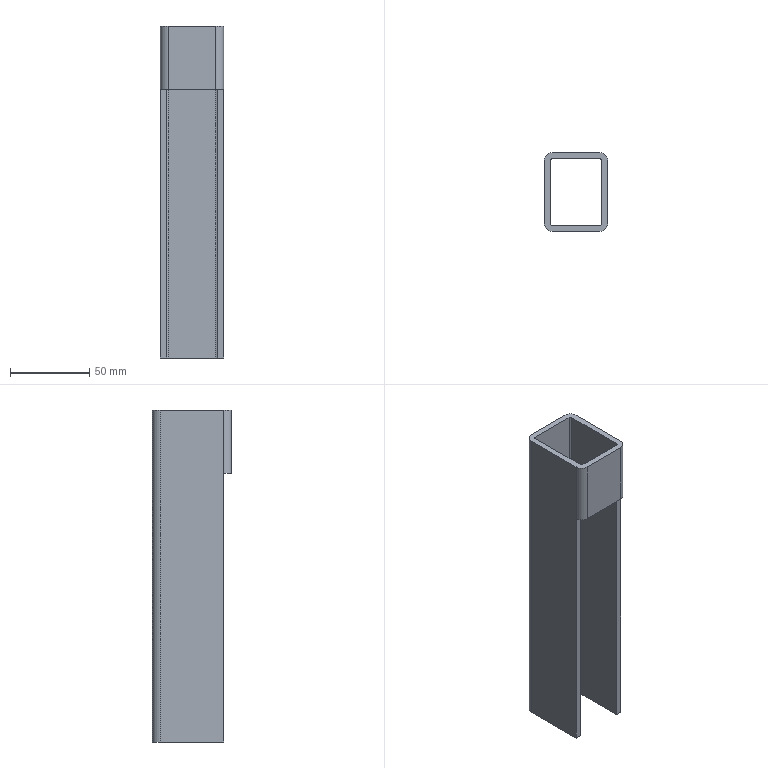Part | SolidWorks | features BaseBody 1 | 1 solid | 21 faces | box 40 x 50 x 210 mm | volume 100329 mm3 | plane 13 | cylinder 8 | commonest cylinder face diameters 2.5 x4 10 x4
STEP:
#1=CARTESIAN_POINT('',(20.,-20.,65.));
#2=VERTEX_POINT('',#1);
#3=CARTESIAN_POINT('',(20.,-20.,-105.));
#4=VERTEX_POINT('',#3);
#5=CARTESIAN_POINT('',(20.,-20.,-115.));
#6=DIRECTION('',(0.,0.,-1.));
#7=VECTOR('',#6,1000.);
#8=LINE('',#5,#7);
#9=EDGE_CURVE('',#2,#4,#8,.T.);
#10=ORIENTED_EDGE('',*,*,#9,.F.);
#11=CARTESIAN_POINT('',(16.25,-20.,65.));
#12=VERTEX_POINT('',#11);
#13=CARTESIAN_POINT('',(20.,-20.,65.));
#14=DIRECTION('',(-1.,0.,0.));
#15=VECTOR('',#14,1000.);
#16=LINE('',#13,#15);
#17=EDGE_CURVE('',#2,#12,#16,.T.);
#18=ORIENTED_EDGE('',*,*,#17,.T.);
#19=CARTESIAN_POINT('',(16.25,-20.,-105.));
#20=VERTEX_POINT('',#19);
#21=CARTESIAN_POINT('',(16.25,-20.,105.));
#22=DIRECTION('',(0.,0.,-1.));
#23=VECTOR('',#22,1000.);
#24=LINE('',#21,#23);
#25=EDGE_CURVE('',#12,#20,#24,.T.);
#26=ORIENTED_EDGE('',*,*,#25,.T.);
#27=CARTESIAN_POINT('',(-15.,-20.,-105.));
#28=DIRECTION('',(-1.,0.,0.));
#29=VECTOR('',#28,1000.);
#30=LINE('',#27,#29);
#31=EDGE_CURVE('',#4,#20,#30,.T.);
#32=ORIENTED_EDGE('',*,*,#31,.F.);
#33=EDGE_LOOP('',(#10,#18,#26,#32));
#34=FACE_OUTER_BOUND('',#33,.T.);
#35=CARTESIAN_POINT('',(20.,-20.,-115.));
#36=DIRECTION('',(0.,1.,0.));
#37=DIRECTION('',(0.,0.,-1.));
#38=AXIS2_PLACEMENT_3D('',#35,#36,#37);
#39=PLANE('',#38);
#40=ADVANCED_FACE('',(#34),#39,.F.);
#41=CARTESIAN_POINT('',(-16.25,-20.,-105.));
#42=VERTEX_POINT('',#41);
#43=CARTESIAN_POINT('',(-16.25,-20.,65.));
#44=VERTEX_POINT('',#43);
#45=CARTESIAN_POINT('',(-16.25,-20.,105.));
#46=DIRECTION('',(0.,0.,1.));
#47=VECTOR('',#46,1000.);
#48=LINE('',#45,#47);
#49=EDGE_CURVE('',#42,#44,#48,.T.);
#50=ORIENTED_EDGE('',*,*,#49,.T.);
#51=CARTESIAN_POINT('',(-20.,-20.,65.));
#52=VERTEX_POINT('',#51);
#53=CARTESIAN_POINT('',(20.,-20.,65.));
#54=DIRECTION('',(-1.,0.,0.));
#55=VECTOR('',#54,1000.);
#56=LINE('',#53,#55);
#57=EDGE_CURVE('',#44,#52,#56,.T.);
#58=ORIENTED_EDGE('',*,*,#57,.T.);
#59=CARTESIAN_POINT('',(-20.,-20.,-105.));
#60=VERTEX_POINT('',#59);
#61=CARTESIAN_POINT('',(-20.,-20.,-115.));
#62=DIRECTION('',(0.,0.,-1.));
#63=VECTOR('',#62,1000.);
#64=LINE('',#61,#63);
#65=EDGE_CURVE('',#52,#60,#64,.T.);
#66=ORIENTED_EDGE('',*,*,#65,.T.);
#67=CARTESIAN_POINT('',(-15.,-20.,-105.));
#68=DIRECTION('',(-1.,0.,0.));
#69=VECTOR('',#68,1000.);
#70=LINE('',#67,#69);
#71=EDGE_CURVE('',#42,#60,#70,.T.);
#72=ORIENTED_EDGE('',*,*,#71,.F.);
#73=EDGE_LOOP('',(#50,#58,#66,#72));
#74=FACE_OUTER_BOUND('',#73,.T.);
#75=CARTESIAN_POINT('',(20.,-20.,-115.));
#76=DIRECTION('',(0.,1.,0.));
#77=DIRECTION('',(0.,0.,-1.));
#78=AXIS2_PLACEMENT_3D('',#75,#76,#77);
#79=PLANE('',#78);
#80=ADVANCED_FACE('',(#74),#79,.F.);
#81=ORIENTED_EDGE('',*,*,#57,.F.);
#82=CARTESIAN_POINT('',(-15.,-21.25,65.));
#83=VERTEX_POINT('',#82);
#84=CARTESIAN_POINT('',(-15.,-20.,65.));
#85=DIRECTION('',(0.,0.,1.));
#86=DIRECTION('',(1.,0.,0.));
#87=AXIS2_PLACEMENT_3D('',#84,#85,#86);
#88=CIRCLE('',#87,1.25);
#89=EDGE_CURVE('',#44,#83,#88,.T.);
#90=ORIENTED_EDGE('',*,*,#89,.T.);
#91=CARTESIAN_POINT('',(15.,-21.25,65.));
#92=VERTEX_POINT('',#91);
#93=CARTESIAN_POINT('',(-15.,-21.25,65.));
#94=DIRECTION('',(1.,0.,0.));
#95=VECTOR('',#94,1000.);
#96=LINE('',#93,#95);
#97=EDGE_CURVE('',#83,#92,#96,.T.);
#98=ORIENTED_EDGE('',*,*,#97,.T.);
#99=CARTESIAN_POINT('',(15.,-20.,65.));
#100=DIRECTION('',(0.,0.,1.));
#101=DIRECTION('',(1.,0.,0.));
#102=AXIS2_PLACEMENT_3D('',#99,#100,#101);
#103=CIRCLE('',#102,1.25);
#104=EDGE_CURVE('',#92,#12,#103,.T.);
#105=ORIENTED_EDGE('',*,*,#104,.T.);
#106=ORIENTED_EDGE('',*,*,#17,.F.);
#107=CARTESIAN_POINT('',(15.,-25.,65.));
#108=VERTEX_POINT('',#107);
#109=CARTESIAN_POINT('',(15.,-20.,65.));
#110=DIRECTION('',(0.,0.,1.));
#111=DIRECTION('',(1.,0.,0.));
#112=AXIS2_PLACEMENT_3D('',#109,#110,#111);
#113=CIRCLE('',#112,5.);
#114=EDGE_CURVE('',#108,#2,#113,.T.);
#115=ORIENTED_EDGE('',*,*,#114,.F.);
#116=CARTESIAN_POINT('',(-15.,-25.,65.));
#117=VERTEX_POINT('',#116);
#118=CARTESIAN_POINT('',(20.,-25.,65.));
#119=DIRECTION('',(-1.,0.,0.));
#120=VECTOR('',#119,1000.);
#121=LINE('',#118,#120);
#122=EDGE_CURVE('',#108,#117,#121,.T.);
#123=ORIENTED_EDGE('',*,*,#122,.T.);
#124=CARTESIAN_POINT('',(-15.,-20.,65.));
#125=DIRECTION('',(0.,0.,1.));
#126=DIRECTION('',(1.,0.,0.));
#127=AXIS2_PLACEMENT_3D('',#124,#125,#126);
#128=CIRCLE('',#127,5.);
#129=EDGE_CURVE('',#52,#117,#128,.T.);
#130=ORIENTED_EDGE('',*,*,#129,.F.);
#131=EDGE_LOOP('',(#81,#90,#98,#105,#106,#115,#123,#130));
#132=FACE_OUTER_BOUND('',#131,.T.);
#133=CARTESIAN_POINT('',(20.,-25.,65.));
#134=DIRECTION('',(0.,0.,1.));
#135=DIRECTION('',(1.,0.,0.));
#136=AXIS2_PLACEMENT_3D('',#133,#134,#135);
#137=PLANE('',#136);
#138=ADVANCED_FACE('',(#132),#137,.F.);
#139=CARTESIAN_POINT('',(15.,21.25,-105.));
#140=VERTEX_POINT('',#139);
#141=CARTESIAN_POINT('',(-15.,21.25,-105.));
#142=VERTEX_POINT('',#141);
#143=CARTESIAN_POINT('',(-15.,21.25,-105.));
#144=DIRECTION('',(-1.,0.,0.));
#145=VECTOR('',#144,1000.);
#146=LINE('',#143,#145);
#147=EDGE_CURVE('',#140,#142,#146,.T.);
#148=ORIENTED_EDGE('',*,*,#147,.F.);
#149=CARTESIAN_POINT('',(15.,21.25,105.));
#150=VERTEX_POINT('',#149);
#151=CARTESIAN_POINT('',(15.,21.25,105.));
#152=DIRECTION('',(0.,0.,-1.));
#153=VECTOR('',#152,1000.);
#154=LINE('',#151,#153);
#155=EDGE_CURVE('',#150,#140,#154,.T.);
#156=ORIENTED_EDGE('',*,*,#155,.F.);
#157=CARTESIAN_POINT('',(-15.,21.25,105.));
#158=VERTEX_POINT('',#157);
#159=CARTESIAN_POINT('',(-15.,21.25,105.));
#160=DIRECTION('',(-1.,0.,0.));
#161=VECTOR('',#160,1000.);
#162=LINE('',#159,#161);
#163=EDGE_CURVE('',#150,#158,#162,.T.);
#164=ORIENTED_EDGE('',*,*,#163,.T.);
#165=CARTESIAN_POINT('',(-15.,21.25,105.));
#166=DIRECTION('',(0.,0.,-1.));
#167=VECTOR('',#166,1000.);
#168=LINE('',#165,#167);
#169=EDGE_CURVE('',#158,#142,#168,.T.);
#170=ORIENTED_EDGE('',*,*,#169,.T.);
#171=EDGE_LOOP('',(#148,#156,#164,#170));
#172=FACE_OUTER_BOUND('',#171,.T.);
#173=CARTESIAN_POINT('',(-15.,21.25,105.));
#174=DIRECTION('',(0.,-1.,0.));
#175=DIRECTION('',(0.,0.,-1.));
#176=AXIS2_PLACEMENT_3D('',#173,#174,#175);
#177=PLANE('',#176);
#178=ADVANCED_FACE('',(#172),#177,.T.);
#179=CARTESIAN_POINT('',(16.25,20.,-105.));
#180=VERTEX_POINT('',#179);
#181=CARTESIAN_POINT('',(15.,20.,-105.));
#182=DIRECTION('',(0.,0.,1.));
#183=DIRECTION('',(-1.,0.,0.));
#184=AXIS2_PLACEMENT_3D('',#181,#182,#183);
#185=CIRCLE('',#184,1.25);
#186=EDGE_CURVE('',#180,#140,#185,.T.);
#187=ORIENTED_EDGE('',*,*,#186,.F.);
#188=CARTESIAN_POINT('',(16.25,20.,105.));
#189=VERTEX_POINT('',#188);
#190=CARTESIAN_POINT('',(16.25,20.,105.));
#191=DIRECTION('',(0.,0.,-1.));
#192=VECTOR('',#191,1000.);
#193=LINE('',#190,#192);
#194=EDGE_CURVE('',#189,#180,#193,.T.);
#195=ORIENTED_EDGE('',*,*,#194,.F.);
#196=CARTESIAN_POINT('',(15.,20.,105.));
#197=DIRECTION('',(0.,0.,1.));
#198=DIRECTION('',(-1.,0.,0.));
#199=AXIS2_PLACEMENT_3D('',#196,#197,#198);
#200=CIRCLE('',#199,1.25);
#201=EDGE_CURVE('',#189,#150,#200,.T.);
#202=ORIENTED_EDGE('',*,*,#201,.T.);
#203=ORIENTED_EDGE('',*,*,#155,.T.);
#204=EDGE_LOOP('',(#187,#195,#202,#203));
#205=FACE_OUTER_BOUND('',#204,.T.);
#206=CARTESIAN_POINT('',(15.,20.,105.));
#207=DIRECTION('',(0.,0.,-1.));
#208=DIRECTION('',(-1.,0.,0.));
#209=AXIS2_PLACEMENT_3D('',#206,#207,#208);
#210=CYLINDRICAL_SURFACE('',#209,1.25);
#211=ADVANCED_FACE('',(#205),#210,.F.);
#212=CARTESIAN_POINT('',(16.25,20.,-105.));
#213=DIRECTION('',(0.,1.,0.));
#214=VECTOR('',#213,1000.);
#215=LINE('',#212,#214);
#216=EDGE_CURVE('',#20,#180,#215,.T.);
#217=ORIENTED_EDGE('',*,*,#216,.F.);
#218=ORIENTED_EDGE('',*,*,#25,.F.);
#219=CARTESIAN_POINT('',(16.25,-20.,105.));
#220=VERTEX_POINT('',#219);
#221=CARTESIAN_POINT('',(16.25,-20.,105.));
#222=DIRECTION('',(0.,0.,-1.));
#223=VECTOR('',#222,1000.);
#224=LINE('',#221,#223);
#225=EDGE_CURVE('',#220,#12,#224,.T.);
#226=ORIENTED_EDGE('',*,*,#225,.F.);
#227=CARTESIAN_POINT('',(16.25,20.,105.));
#228=DIRECTION('',(0.,1.,0.));
#229=VECTOR('',#228,1000.);
#230=LINE('',#227,#229);
#231=EDGE_CURVE('',#220,#189,#230,.T.);
#232=ORIENTED_EDGE('',*,*,#231,.T.);
#233=ORIENTED_EDGE('',*,*,#194,.T.);
#234=EDGE_LOOP('',(#217,#218,#226,#232,#233));
#235=FACE_OUTER_BOUND('',#234,.T.);
#236=CARTESIAN_POINT('',(16.25,20.,105.));
#237=DIRECTION('',(-1.,0.,0.));
#238=DIRECTION('',(0.,1.,0.));
#239=AXIS2_PLACEMENT_3D('',#236,#237,#238);
#240=PLANE('',#239);
#241=ADVANCED_FACE('',(#235),#240,.T.);
#242=ORIENTED_EDGE('',*,*,#104,.F.);
#243=CARTESIAN_POINT('',(15.,-21.25,105.));
#244=VERTEX_POINT('',#243);
#245=CARTESIAN_POINT('',(15.,-21.25,105.));
#246=DIRECTION('',(0.,0.,-1.));
#247=VECTOR('',#246,1000.);
#248=LINE('',#245,#247);
#249=EDGE_CURVE('',#244,#92,#248,.T.);
#250=ORIENTED_EDGE('',*,*,#249,.F.);
#251=CARTESIAN_POINT('',(15.,-20.,105.));
#252=DIRECTION('',(0.,0.,1.));
#253=DIRECTION('',(1.,0.,0.));
#254=AXIS2_PLACEMENT_3D('',#251,#252,#253);
#255=CIRCLE('',#254,1.25);
#256=EDGE_CURVE('',#244,#220,#255,.T.);
#257=ORIENTED_EDGE('',*,*,#256,.T.);
#258=ORIENTED_EDGE('',*,*,#225,.T.);
#259=EDGE_LOOP('',(#242,#250,#257,#258));
#260=FACE_OUTER_BOUND('',#259,.T.);
#261=CARTESIAN_POINT('',(15.,-20.,105.));
#262=DIRECTION('',(0.,0.,-1.));
#263=DIRECTION('',(-1.,0.,0.));
#264=AXIS2_PLACEMENT_3D('',#261,#262,#263);
#265=CYLINDRICAL_SURFACE('',#264,1.25);
#266=ADVANCED_FACE('',(#260),#265,.F.);
#267=ORIENTED_EDGE('',*,*,#97,.F.);
#268=CARTESIAN_POINT('',(-15.,-21.25,105.));
#269=VERTEX_POINT('',#268);
#270=CARTESIAN_POINT('',(-15.,-21.25,105.));
#271=DIRECTION('',(0.,0.,-1.));
#272=VECTOR('',#271,1000.);
#273=LINE('',#270,#272);
#274=EDGE_CURVE('',#269,#83,#273,.T.);
#275=ORIENTED_EDGE('',*,*,#274,.F.);
#276=CARTESIAN_POINT('',(-15.,-21.25,105.));
#277=DIRECTION('',(1.,0.,0.));
#278=VECTOR('',#277,1000.);
#279=LINE('',#276,#278);
#280=EDGE_CURVE('',#269,#244,#279,.T.);
#281=ORIENTED_EDGE('',*,*,#280,.T.);
#282=ORIENTED_EDGE('',*,*,#249,.T.);
#283=EDGE_LOOP('',(#267,#275,#281,#282));
#284=FACE_OUTER_BOUND('',#283,.T.);
#285=CARTESIAN_POINT('',(-15.,-21.25,105.));
#286=DIRECTION('',(0.,1.,0.));
#287=DIRECTION('',(1.,0.,0.));
#288=AXIS2_PLACEMENT_3D('',#285,#286,#287);
#289=PLANE('',#288);
#290=ADVANCED_FACE('',(#284),#289,.T.);
#291=ORIENTED_EDGE('',*,*,#89,.F.);
#292=CARTESIAN_POINT('',(-16.25,-20.,105.));
#293=VERTEX_POINT('',#292);
#294=CARTESIAN_POINT('',(-16.25,-20.,105.));
#295=DIRECTION('',(0.,0.,-1.));
#296=VECTOR('',#295,1000.);
#297=LINE('',#294,#296);
#298=EDGE_CURVE('',#293,#44,#297,.T.);
#299=ORIENTED_EDGE('',*,*,#298,.F.);
#300=CARTESIAN_POINT('',(-15.,-20.,105.));
#301=DIRECTION('',(0.,0.,1.));
#302=DIRECTION('',(1.,0.,0.));
#303=AXIS2_PLACEMENT_3D('',#300,#301,#302);
#304=CIRCLE('',#303,1.25);
#305=EDGE_CURVE('',#293,#269,#304,.T.);
#306=ORIENTED_EDGE('',*,*,#305,.T.);
#307=ORIENTED_EDGE('',*,*,#274,.T.);
#308=EDGE_LOOP('',(#291,#299,#306,#307));
#309=FACE_OUTER_BOUND('',#308,.T.);
#310=CARTESIAN_POINT('',(-15.,-20.,105.));
#311=DIRECTION('',(0.,0.,-1.));
#312=DIRECTION('',(-1.,0.,0.));
#313=AXIS2_PLACEMENT_3D('',#310,#311,#312);
#314=CYLINDRICAL_SURFACE('',#313,1.25);
#315=ADVANCED_FACE('',(#309),#314,.F.);
#316=CARTESIAN_POINT('',(-16.25,20.,-105.));
#317=VERTEX_POINT('',#316);
#318=CARTESIAN_POINT('',(-16.25,20.,-105.));
#319=DIRECTION('',(0.,-1.,0.));
#320=VECTOR('',#319,1000.);
#321=LINE('',#318,#320);
#322=EDGE_CURVE('',#317,#42,#321,.T.);
#323=ORIENTED_EDGE('',*,*,#322,.F.);
#324=CARTESIAN_POINT('',(-16.25,20.,105.));
#325=VERTEX_POINT('',#324);
#326=CARTESIAN_POINT('',(-16.25,20.,105.));
#327=DIRECTION('',(0.,0.,-1.));
#328=VECTOR('',#327,1000.);
#329=LINE('',#326,#328);
#330=EDGE_CURVE('',#325,#317,#329,.T.);
#331=ORIENTED_EDGE('',*,*,#330,.F.);
#332=CARTESIAN_POINT('',(-16.25,20.,105.));
#333=DIRECTION('',(0.,-1.,0.));
#334=VECTOR('',#333,1000.);
#335=LINE('',#332,#334);
#336=EDGE_CURVE('',#325,#293,#335,.T.);
#337=ORIENTED_EDGE('',*,*,#336,.T.);
#338=ORIENTED_EDGE('',*,*,#298,.T.);
#339=ORIENTED_EDGE('',*,*,#49,.F.);
#340=EDGE_LOOP('',(#323,#331,#337,#338,#339));
#341=FACE_OUTER_BOUND('',#340,.T.);
#342=CARTESIAN_POINT('',(-16.25,20.,105.));
#343=DIRECTION('',(1.,0.,0.));
#344=DIRECTION('',(0.,1.,0.));
#345=AXIS2_PLACEMENT_3D('',#342,#343,#344);
#346=PLANE('',#345);
#347=ADVANCED_FACE('',(#341),#346,.T.);
#348=CARTESIAN_POINT('',(-15.,20.,-105.));
#349=DIRECTION('',(0.,0.,1.));
#350=DIRECTION('',(1.,0.,0.));
#351=AXIS2_PLACEMENT_3D('',#348,#349,#350);
#352=CIRCLE('',#351,1.25);
#353=EDGE_CURVE('',#142,#317,#352,.T.);
#354=ORIENTED_EDGE('',*,*,#353,.F.);
#355=ORIENTED_EDGE('',*,*,#169,.F.);
#356=CARTESIAN_POINT('',(-15.,20.,105.));
#357=DIRECTION('',(0.,0.,1.));
#358=DIRECTION('',(1.,0.,0.));
#359=AXIS2_PLACEMENT_3D('',#356,#357,#358);
#360=CIRCLE('',#359,1.25);
#361=EDGE_CURVE('',#158,#325,#360,.T.);
#362=ORIENTED_EDGE('',*,*,#361,.T.);
#363=ORIENTED_EDGE('',*,*,#330,.T.);
#364=EDGE_LOOP('',(#354,#355,#362,#363));
#365=FACE_OUTER_BOUND('',#364,.T.);
#366=CARTESIAN_POINT('',(-15.,20.,105.));
#367=DIRECTION('',(0.,0.,-1.));
#368=DIRECTION('',(-1.,0.,0.));
#369=AXIS2_PLACEMENT_3D('',#366,#367,#368);
#370=CYLINDRICAL_SURFACE('',#369,1.25);
#371=ADVANCED_FACE('',(#365),#370,.F.);
#372=CARTESIAN_POINT('',(-20.,20.,-105.));
#373=VERTEX_POINT('',#372);
#374=CARTESIAN_POINT('',(-20.,20.,-105.));
#375=DIRECTION('',(0.,-1.,0.));
#376=VECTOR('',#375,1000.);
#377=LINE('',#374,#376);
#378=EDGE_CURVE('',#373,#60,#377,.T.);
#379=ORIENTED_EDGE('',*,*,#378,.T.);
#380=ORIENTED_EDGE('',*,*,#65,.F.);
#381=CARTESIAN_POINT('',(-20.,-20.,105.));
#382=VERTEX_POINT('',#381);
#383=CARTESIAN_POINT('',(-20.,-20.,105.));
#384=DIRECTION('',(0.,0.,-1.));
#385=VECTOR('',#384,1000.);
#386=LINE('',#383,#385);
#387=EDGE_CURVE('',#382,#52,#386,.T.);
#388=ORIENTED_EDGE('',*,*,#387,.F.);
#389=CARTESIAN_POINT('',(-20.,20.,105.));
#390=VERTEX_POINT('',#389);
#391=CARTESIAN_POINT('',(-20.,20.,105.));
#392=DIRECTION('',(0.,-1.,0.));
#393=VECTOR('',#392,1000.);
#394=LINE('',#391,#393);
#395=EDGE_CURVE('',#390,#382,#394,.T.);
#396=ORIENTED_EDGE('',*,*,#395,.F.);
#397=CARTESIAN_POINT('',(-20.,20.,105.));
#398=DIRECTION('',(0.,0.,-1.));
#399=VECTOR('',#398,1000.);
#400=LINE('',#397,#399);
#401=EDGE_CURVE('',#390,#373,#400,.T.);
#402=ORIENTED_EDGE('',*,*,#401,.T.);
#403=EDGE_LOOP('',(#379,#380,#388,#396,#402));
#404=FACE_OUTER_BOUND('',#403,.T.);
#405=CARTESIAN_POINT('',(-20.,20.,105.));
#406=DIRECTION('',(1.,0.,0.));
#407=DIRECTION('',(0.,1.,0.));
#408=AXIS2_PLACEMENT_3D('',#405,#406,#407);
#409=PLANE('',#408);
#410=ADVANCED_FACE('',(#404),#409,.F.);
#411=CARTESIAN_POINT('',(-15.,25.,-105.));
#412=VERTEX_POINT('',#411);
#413=CARTESIAN_POINT('',(-15.,20.,-105.));
#414=DIRECTION('',(0.,0.,1.));
#415=DIRECTION('',(1.,0.,0.));
#416=AXIS2_PLACEMENT_3D('',#413,#414,#415);
#417=CIRCLE('',#416,5.);
#418=EDGE_CURVE('',#412,#373,#417,.T.);
#419=ORIENTED_EDGE('',*,*,#418,.T.);
#420=ORIENTED_EDGE('',*,*,#401,.F.);
#421=CARTESIAN_POINT('',(-15.,25.,105.));
#422=VERTEX_POINT('',#421);
#423=CARTESIAN_POINT('',(-15.,20.,105.));
#424=DIRECTION('',(0.,0.,1.));
#425=DIRECTION('',(1.,0.,0.));
#426=AXIS2_PLACEMENT_3D('',#423,#424,#425);
#427=CIRCLE('',#426,5.);
#428=EDGE_CURVE('',#422,#390,#427,.T.);
#429=ORIENTED_EDGE('',*,*,#428,.F.);
#430=CARTESIAN_POINT('',(-15.,25.,105.));
#431=DIRECTION('',(0.,0.,-1.));
#432=VECTOR('',#431,1000.);
#433=LINE('',#430,#432);
#434=EDGE_CURVE('',#422,#412,#433,.T.);
#435=ORIENTED_EDGE('',*,*,#434,.T.);
#436=EDGE_LOOP('',(#419,#420,#429,#435));
#437=FACE_OUTER_BOUND('',#436,.T.);
#438=CARTESIAN_POINT('',(-15.,20.,105.));
#439=DIRECTION('',(0.,0.,-1.));
#440=DIRECTION('',(-1.,0.,0.));
#441=AXIS2_PLACEMENT_3D('',#438,#439,#440);
#442=CYLINDRICAL_SURFACE('',#441,5.);
#443=ADVANCED_FACE('',(#437),#442,.T.);
#444=CARTESIAN_POINT('',(15.,25.,-105.));
#445=VERTEX_POINT('',#444);
#446=CARTESIAN_POINT('',(-15.,25.,-105.));
#447=DIRECTION('',(-1.,0.,0.));
#448=VECTOR('',#447,1000.);
#449=LINE('',#446,#448);
#450=EDGE_CURVE('',#445,#412,#449,.T.);
#451=ORIENTED_EDGE('',*,*,#450,.T.);
#452=ORIENTED_EDGE('',*,*,#434,.F.);
#453=CARTESIAN_POINT('',(15.,25.,105.));
#454=VERTEX_POINT('',#453);
#455=CARTESIAN_POINT('',(-15.,25.,105.));
#456=DIRECTION('',(-1.,0.,0.));
#457=VECTOR('',#456,1000.);
#458=LINE('',#455,#457);
#459=EDGE_CURVE('',#454,#422,#458,.T.);
#460=ORIENTED_EDGE('',*,*,#459,.F.);
#461=CARTESIAN_POINT('',(15.,25.,105.));
#462=DIRECTION('',(0.,0.,-1.));
#463=VECTOR('',#462,1000.);
#464=LINE('',#461,#463);
#465=EDGE_CURVE('',#454,#445,#464,.T.);
#466=ORIENTED_EDGE('',*,*,#465,.T.);
#467=EDGE_LOOP('',(#451,#452,#460,#466));
#468=FACE_OUTER_BOUND('',#467,.T.);
#469=CARTESIAN_POINT('',(-15.,25.,105.));
#470=DIRECTION('',(0.,-1.,0.));
#471=DIRECTION('',(0.,0.,-1.));
#472=AXIS2_PLACEMENT_3D('',#469,#470,#471);
#473=PLANE('',#472);
#474=ADVANCED_FACE('',(#468),#473,.F.);
#475=CARTESIAN_POINT('',(20.,20.,-105.));
#476=VERTEX_POINT('',#475);
#477=CARTESIAN_POINT('',(15.,20.,-105.));
#478=DIRECTION('',(0.,0.,1.));
#479=DIRECTION('',(-1.,0.,0.));
#480=AXIS2_PLACEMENT_3D('',#477,#478,#479);
#481=CIRCLE('',#480,5.);
#482=EDGE_CURVE('',#476,#445,#481,.T.);
#483=ORIENTED_EDGE('',*,*,#482,.T.);
#484=ORIENTED_EDGE('',*,*,#465,.F.);
#485=CARTESIAN_POINT('',(20.,20.,105.));
#486=VERTEX_POINT('',#485);
#487=CARTESIAN_POINT('',(15.,20.,105.));
#488=DIRECTION('',(0.,0.,1.));
#489=DIRECTION('',(-1.,0.,0.));
#490=AXIS2_PLACEMENT_3D('',#487,#488,#489);
#491=CIRCLE('',#490,5.);
#492=EDGE_CURVE('',#486,#454,#491,.T.);
#493=ORIENTED_EDGE('',*,*,#492,.F.);
#494=CARTESIAN_POINT('',(20.,20.,105.));
#495=DIRECTION('',(0.,0.,-1.));
#496=VECTOR('',#495,1000.);
#497=LINE('',#494,#496);
#498=EDGE_CURVE('',#486,#476,#497,.T.);
#499=ORIENTED_EDGE('',*,*,#498,.T.);
#500=EDGE_LOOP('',(#483,#484,#493,#499));
#501=FACE_OUTER_BOUND('',#500,.T.);
#502=CARTESIAN_POINT('',(15.,20.,105.));
#503=DIRECTION('',(0.,0.,-1.));
#504=DIRECTION('',(-1.,0.,0.));
#505=AXIS2_PLACEMENT_3D('',#502,#503,#504);
#506=CYLINDRICAL_SURFACE('',#505,5.);
#507=ADVANCED_FACE('',(#501),#506,.T.);
#508=CARTESIAN_POINT('',(20.,20.,-105.));
#509=DIRECTION('',(0.,1.,0.));
#510=VECTOR('',#509,1000.);
#511=LINE('',#508,#510);
#512=EDGE_CURVE('',#4,#476,#511,.T.);
#513=ORIENTED_EDGE('',*,*,#512,.T.);
#514=ORIENTED_EDGE('',*,*,#498,.F.);
#515=CARTESIAN_POINT('',(20.,-20.,105.));
#516=VERTEX_POINT('',#515);
#517=CARTESIAN_POINT('',(20.,20.,105.));
#518=DIRECTION('',(0.,1.,0.));
#519=VECTOR('',#518,1000.);
#520=LINE('',#517,#519);
#521=EDGE_CURVE('',#516,#486,#520,.T.);
#522=ORIENTED_EDGE('',*,*,#521,.F.);
#523=CARTESIAN_POINT('',(20.,-20.,105.));
#524=DIRECTION('',(0.,0.,-1.));
#525=VECTOR('',#524,1000.);
#526=LINE('',#523,#525);
#527=EDGE_CURVE('',#516,#2,#526,.T.);
#528=ORIENTED_EDGE('',*,*,#527,.T.);
#529=ORIENTED_EDGE('',*,*,#9,.T.);
#530=EDGE_LOOP('',(#513,#514,#522,#528,#529));
#531=FACE_OUTER_BOUND('',#530,.T.);
#532=CARTESIAN_POINT('',(20.,20.,105.));
#533=DIRECTION('',(-1.,0.,0.));
#534=DIRECTION('',(0.,1.,0.));
#535=AXIS2_PLACEMENT_3D('',#532,#533,#534);
#536=PLANE('',#535);
#537=ADVANCED_FACE('',(#531),#536,.F.);
#538=CARTESIAN_POINT('',(15.,-25.,105.));
#539=VERTEX_POINT('',#538);
#540=CARTESIAN_POINT('',(15.,-25.,105.));
#541=DIRECTION('',(0.,0.,-1.));
#542=VECTOR('',#541,1000.);
#543=LINE('',#540,#542);
#544=EDGE_CURVE('',#539,#108,#543,.T.);
#545=ORIENTED_EDGE('',*,*,#544,.T.);
#546=ORIENTED_EDGE('',*,*,#114,.T.);
#547=ORIENTED_EDGE('',*,*,#527,.F.);
#548=CARTESIAN_POINT('',(15.,-20.,105.));
#549=DIRECTION('',(0.,0.,1.));
#550=DIRECTION('',(1.,0.,0.));
#551=AXIS2_PLACEMENT_3D('',#548,#549,#550);
#552=CIRCLE('',#551,5.);
#553=EDGE_CURVE('',#539,#516,#552,.T.);
#554=ORIENTED_EDGE('',*,*,#553,.F.);
#555=EDGE_LOOP('',(#545,#546,#547,#554));
#556=FACE_OUTER_BOUND('',#555,.T.);
#557=CARTESIAN_POINT('',(15.,-20.,105.));
#558=DIRECTION('',(0.,0.,-1.));
#559=DIRECTION('',(-1.,0.,0.));
#560=AXIS2_PLACEMENT_3D('',#557,#558,#559);
#561=CYLINDRICAL_SURFACE('',#560,5.);
#562=ADVANCED_FACE('',(#556),#561,.T.);
#563=CARTESIAN_POINT('',(-15.,-25.,105.));
#564=VERTEX_POINT('',#563);
#565=CARTESIAN_POINT('',(-15.,-25.,105.));
#566=DIRECTION('',(0.,0.,-1.));
#567=VECTOR('',#566,1000.);
#568=LINE('',#565,#567);
#569=EDGE_CURVE('',#564,#117,#568,.T.);
#570=ORIENTED_EDGE('',*,*,#569,.T.);
#571=ORIENTED_EDGE('',*,*,#122,.F.);
#572=ORIENTED_EDGE('',*,*,#544,.F.);
#573=CARTESIAN_POINT('',(-15.,-25.,105.));
#574=DIRECTION('',(1.,0.,0.));
#575=VECTOR('',#574,1000.);
#576=LINE('',#573,#575);
#577=EDGE_CURVE('',#564,#539,#576,.T.);
#578=ORIENTED_EDGE('',*,*,#577,.F.);
#579=EDGE_LOOP('',(#570,#571,#572,#578));
#580=FACE_OUTER_BOUND('',#579,.T.);
#581=CARTESIAN_POINT('',(-15.,-25.,105.));
#582=DIRECTION('',(0.,1.,0.));
#583=DIRECTION('',(1.,0.,0.));
#584=AXIS2_PLACEMENT_3D('',#581,#582,#583);
#585=PLANE('',#584);
#586=ADVANCED_FACE('',(#580),#585,.F.);
#587=ORIENTED_EDGE('',*,*,#387,.T.);
#588=ORIENTED_EDGE('',*,*,#129,.T.);
#589=ORIENTED_EDGE('',*,*,#569,.F.);
#590=CARTESIAN_POINT('',(-15.,-20.,105.));
#591=DIRECTION('',(0.,0.,1.));
#592=DIRECTION('',(1.,0.,0.));
#593=AXIS2_PLACEMENT_3D('',#590,#591,#592);
#594=CIRCLE('',#593,5.);
#595=EDGE_CURVE('',#382,#564,#594,.T.);
#596=ORIENTED_EDGE('',*,*,#595,.F.);
#597=EDGE_LOOP('',(#587,#588,#589,#596));
#598=FACE_OUTER_BOUND('',#597,.T.);
#599=CARTESIAN_POINT('',(-15.,-20.,105.));
#600=DIRECTION('',(0.,0.,-1.));
#601=DIRECTION('',(-1.,0.,0.));
#602=AXIS2_PLACEMENT_3D('',#599,#600,#601);
#603=CYLINDRICAL_SURFACE('',#602,5.);
#604=ADVANCED_FACE('',(#598),#603,.T.);
#605=ORIENTED_EDGE('',*,*,#512,.F.);
#606=ORIENTED_EDGE('',*,*,#31,.T.);
#607=ORIENTED_EDGE('',*,*,#216,.T.);
#608=ORIENTED_EDGE('',*,*,#186,.T.);
#609=ORIENTED_EDGE('',*,*,#147,.T.);
#610=ORIENTED_EDGE('',*,*,#353,.T.);
#611=ORIENTED_EDGE('',*,*,#322,.T.);
#612=ORIENTED_EDGE('',*,*,#71,.T.);
#613=ORIENTED_EDGE('',*,*,#378,.F.);
#614=ORIENTED_EDGE('',*,*,#418,.F.);
#615=ORIENTED_EDGE('',*,*,#450,.F.);
#616=ORIENTED_EDGE('',*,*,#482,.F.);
#617=EDGE_LOOP('',(#605,#606,#607,#608,#609,#610,#611,#612,#613,#614,#615,#616));
#618=FACE_OUTER_BOUND('',#617,.T.);
#619=CARTESIAN_POINT('',(-15.,-20.,-105.));
#620=DIRECTION('',(0.,0.,1.));
#621=DIRECTION('',(1.,0.,0.));
#622=AXIS2_PLACEMENT_3D('',#619,#620,#621);
#623=PLANE('',#622);
#624=ADVANCED_FACE('',(#618),#623,.F.);
#625=ORIENTED_EDGE('',*,*,#336,.F.);
#626=ORIENTED_EDGE('',*,*,#361,.F.);
#627=ORIENTED_EDGE('',*,*,#163,.F.);
#628=ORIENTED_EDGE('',*,*,#201,.F.);
#629=ORIENTED_EDGE('',*,*,#231,.F.);
#630=ORIENTED_EDGE('',*,*,#256,.F.);
#631=ORIENTED_EDGE('',*,*,#280,.F.);
#632=ORIENTED_EDGE('',*,*,#305,.F.);
#633=EDGE_LOOP('',(#625,#626,#627,#628,#629,#630,#631,#632));
#634=FACE_BOUND('',#633,.T.);
#635=ORIENTED_EDGE('',*,*,#595,.T.);
#636=ORIENTED_EDGE('',*,*,#577,.T.);
#637=ORIENTED_EDGE('',*,*,#553,.T.);
#638=ORIENTED_EDGE('',*,*,#521,.T.);
#639=ORIENTED_EDGE('',*,*,#492,.T.);
#640=ORIENTED_EDGE('',*,*,#459,.T.);
#641=ORIENTED_EDGE('',*,*,#428,.T.);
#642=ORIENTED_EDGE('',*,*,#395,.T.);
#643=EDGE_LOOP('',(#635,#636,#637,#638,#639,#640,#641,#642));
#644=FACE_OUTER_BOUND('',#643,.T.);
#645=CARTESIAN_POINT('',(-15.,-20.,105.));
#646=DIRECTION('',(0.,0.,1.));
#647=DIRECTION('',(1.,0.,0.));
#648=AXIS2_PLACEMENT_3D('',#645,#646,#647);
#649=PLANE('',#648);
#650=ADVANCED_FACE('',(#634,#644),#649,.T.);
#651=CLOSED_SHELL('',(#40,#80,#138,#178,#211,#241,#266,#290,#315,#347,#371,#410,#443,#474,#507,#537,#562,#586,#604,#624,#650));
#652=MANIFOLD_SOLID_BREP('',#651);
#653=CARTESIAN_POINT('',(0.,0.,0.));
#654=DIRECTION('',(0.,0.,1.));
#655=DIRECTION('',(1.,0.,0.));
#656=AXIS2_PLACEMENT_3D('',#653,#654,#655);
#657=(LENGTH_UNIT()NAMED_UNIT(*)SI_UNIT(.MILLI.,.METRE.));
#658=UNCERTAINTY_MEASURE_WITH_UNIT(LENGTH_MEASURE(0.00001),#657,'','');
#659=(NAMED_UNIT(*)PLANE_ANGLE_UNIT()SI_UNIT($,.RADIAN.));
#660=(NAMED_UNIT(*)SI_UNIT($,.STERADIAN.)SOLID_ANGLE_UNIT());
#661=(GEOMETRIC_REPRESENTATION_CONTEXT(3)GLOBAL_UNCERTAINTY_ASSIGNED_CONTEXT((#658))GLOBAL_UNIT_ASSIGNED_CONTEXT((#657,#659,#660))REPRESENTATION_CONTEXT('',''));
#662=ADVANCED_BREP_SHAPE_REPRESENTATION('',(#652,#656),#661);